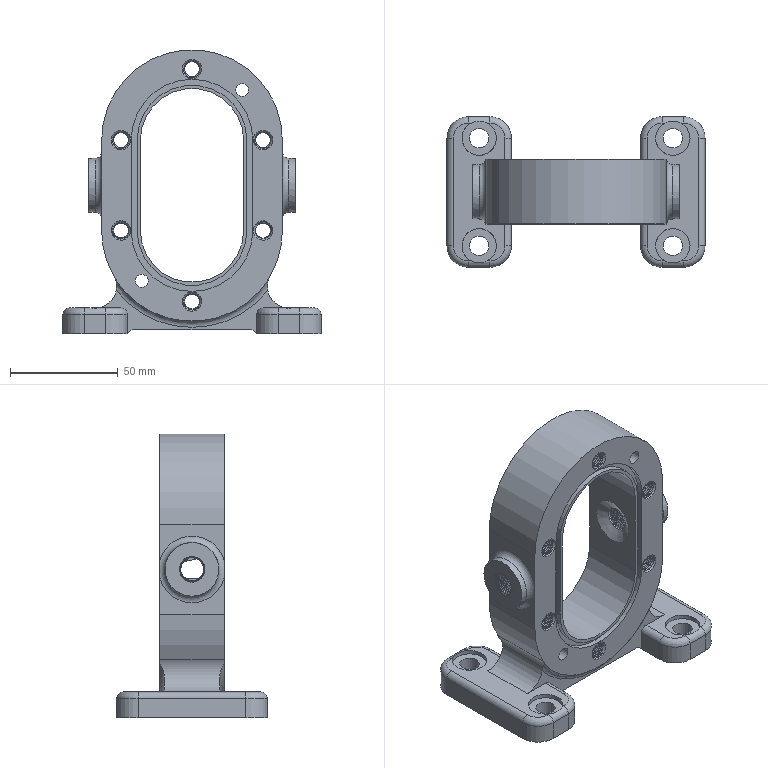Part | NX | features EXTRUDE 12, THREADS 8, DATUM_CSYS 7, DATUM_PLANE 6, EXTRACT_STRING 6, SKETCH 6, BLEND 5, CHAMFER 4, EXTRACT_FACE 4, Instance Feature 2, Mirror Feature 2 | 1 solid | 160 faces | box 120 x 70 x 132 mm | volume 199459 mm3 | cylinder 63 | plane 51 | cone 18 | spline 16 | torus 12 | commonest cylinder face diameters 6 x14 20 x10 7 x6 8 x6 9 x4 16 x4